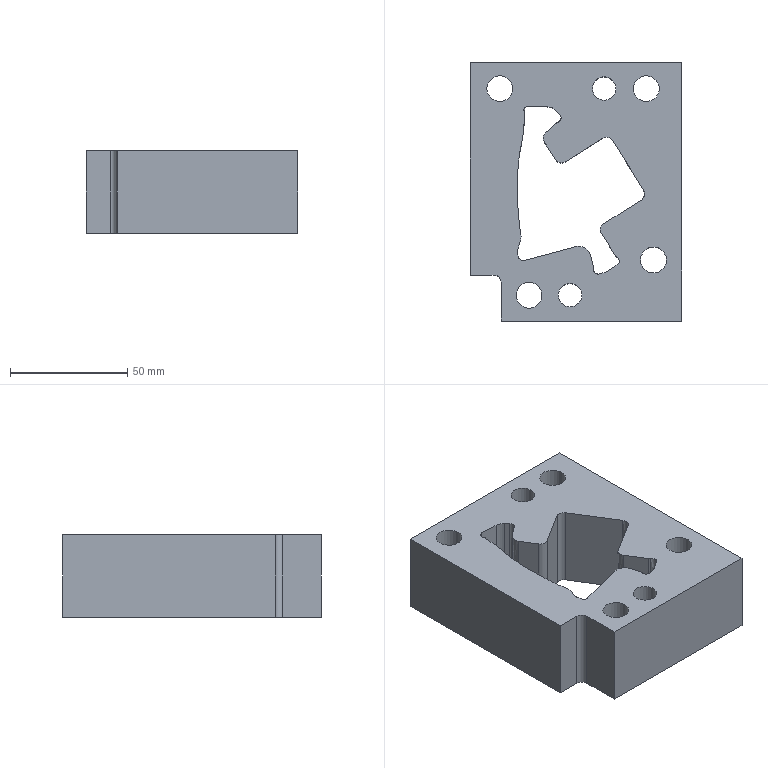Part | NX | features solid 2 | 1 solid | 64 faces | box 90 x 110 x 35 mm | volume 231539 mm3 | cylinder 22 | spline 22 | plane 20 | commonest cylinder face diameters 10 x6 11 x6 17 x4 6 x3 4 x2 200 x1